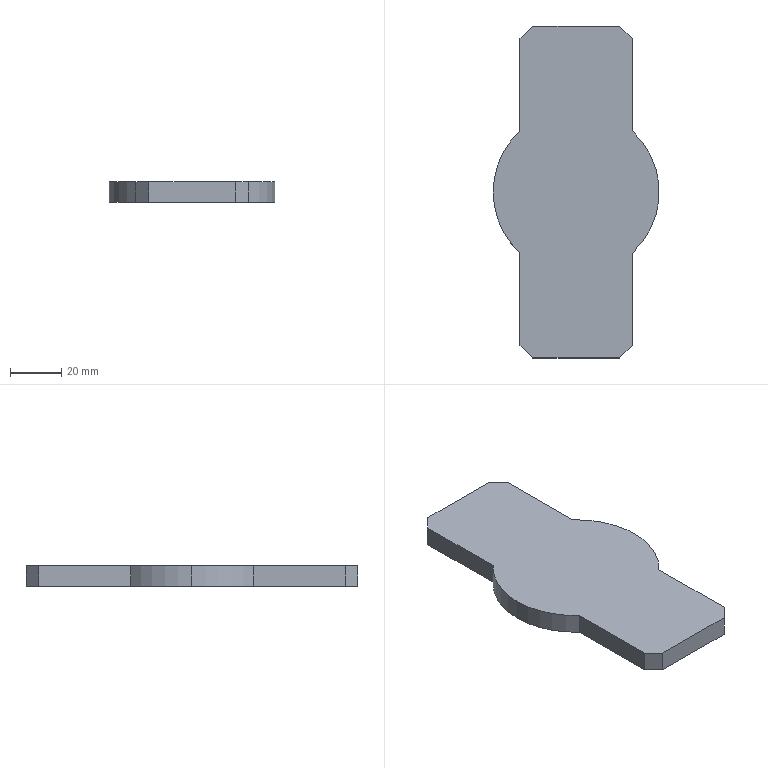Part | SolidWorks | features Chamfer 1, Extrusion 1, ICE 1 | 1 solid | 15 faces | box 65 x 130 x 8 mm | volume 50920 mm3 | plane 12 | cylinder 3 | commonest cylinder face diameters 65 x3
STEP:
#1=CARTESIAN_POINT('',(-32.5,0.,4.));
#2=VERTEX_POINT('',#1);
#3=CARTESIAN_POINT('',(-22.,-23.922,4.));
#4=VERTEX_POINT('',#3);
#5=CARTESIAN_POINT('',(0.,0.,4.));
#6=DIRECTION('',(0.,0.,1.));
#7=DIRECTION('',(1.,0.,0.));
#8=AXIS2_PLACEMENT_3D('',#5,#6,#7);
#9=CIRCLE('',#8,32.5);
#10=EDGE_CURVE('',#2,#4,#9,.T.);
#11=ORIENTED_EDGE('',*,*,#10,.F.);
#12=CARTESIAN_POINT('',(-32.5,0.,-4.));
#13=VERTEX_POINT('',#12);
#14=CARTESIAN_POINT('',(-32.5,0.,4.));
#15=DIRECTION('',(0.,0.,-1.));
#16=VECTOR('',#15,1000.);
#17=LINE('',#14,#16);
#18=EDGE_CURVE('',#2,#13,#17,.T.);
#19=ORIENTED_EDGE('',*,*,#18,.T.);
#20=CARTESIAN_POINT('',(-22.,-23.922,-4.));
#21=VERTEX_POINT('',#20);
#22=CARTESIAN_POINT('',(0.,0.,-4.));
#23=DIRECTION('',(0.,0.,1.));
#24=DIRECTION('',(1.,0.,0.));
#25=AXIS2_PLACEMENT_3D('',#22,#23,#24);
#26=CIRCLE('',#25,32.5);
#27=EDGE_CURVE('',#13,#21,#26,.T.);
#28=ORIENTED_EDGE('',*,*,#27,.T.);
#29=CARTESIAN_POINT('',(-22.,-23.922,4.));
#30=DIRECTION('',(0.,0.,1.));
#31=VECTOR('',#30,1000.);
#32=LINE('',#29,#31);
#33=EDGE_CURVE('',#21,#4,#32,.T.);
#34=ORIENTED_EDGE('',*,*,#33,.T.);
#35=EDGE_LOOP('',(#11,#19,#28,#34));
#36=FACE_OUTER_BOUND('',#35,.T.);
#37=CARTESIAN_POINT('',(0.,0.,4.));
#38=DIRECTION('',(0.,0.,-1.));
#39=DIRECTION('',(-1.,0.,0.));
#40=AXIS2_PLACEMENT_3D('',#37,#38,#39);
#41=CYLINDRICAL_SURFACE('',#40,32.5);
#42=ADVANCED_FACE('',(#36),#41,.T.);
#43=CARTESIAN_POINT('',(22.,-23.922,4.));
#44=VERTEX_POINT('',#43);
#45=CARTESIAN_POINT('',(22.,23.922,4.));
#46=VERTEX_POINT('',#45);
#47=CARTESIAN_POINT('',(0.,0.,4.));
#48=DIRECTION('',(0.,0.,1.));
#49=DIRECTION('',(1.,0.,0.));
#50=AXIS2_PLACEMENT_3D('',#47,#48,#49);
#51=CIRCLE('',#50,32.5);
#52=EDGE_CURVE('',#44,#46,#51,.T.);
#53=ORIENTED_EDGE('',*,*,#52,.F.);
#54=CARTESIAN_POINT('',(22.,-23.922,-4.));
#55=VERTEX_POINT('',#54);
#56=CARTESIAN_POINT('',(22.,-23.922,4.));
#57=DIRECTION('',(0.,0.,-1.));
#58=VECTOR('',#57,1000.);
#59=LINE('',#56,#58);
#60=EDGE_CURVE('',#44,#55,#59,.T.);
#61=ORIENTED_EDGE('',*,*,#60,.T.);
#62=CARTESIAN_POINT('',(22.,23.922,-4.));
#63=VERTEX_POINT('',#62);
#64=CARTESIAN_POINT('',(0.,0.,-4.));
#65=DIRECTION('',(0.,0.,1.));
#66=DIRECTION('',(1.,0.,0.));
#67=AXIS2_PLACEMENT_3D('',#64,#65,#66);
#68=CIRCLE('',#67,32.5);
#69=EDGE_CURVE('',#55,#63,#68,.T.);
#70=ORIENTED_EDGE('',*,*,#69,.T.);
#71=CARTESIAN_POINT('',(22.,23.922,4.));
#72=DIRECTION('',(0.,0.,1.));
#73=VECTOR('',#72,1000.);
#74=LINE('',#71,#73);
#75=EDGE_CURVE('',#63,#46,#74,.T.);
#76=ORIENTED_EDGE('',*,*,#75,.T.);
#77=EDGE_LOOP('',(#53,#61,#70,#76));
#78=FACE_OUTER_BOUND('',#77,.T.);
#79=CARTESIAN_POINT('',(0.,0.,4.));
#80=DIRECTION('',(0.,0.,-1.));
#81=DIRECTION('',(-1.,0.,0.));
#82=AXIS2_PLACEMENT_3D('',#79,#80,#81);
#83=CYLINDRICAL_SURFACE('',#82,32.5);
#84=ADVANCED_FACE('',(#78),#83,.T.);
#85=ORIENTED_EDGE('',*,*,#18,.F.);
#86=CARTESIAN_POINT('',(-22.,23.922,4.));
#87=VERTEX_POINT('',#86);
#88=CARTESIAN_POINT('',(0.,0.,4.));
#89=DIRECTION('',(0.,0.,1.));
#90=DIRECTION('',(1.,0.,0.));
#91=AXIS2_PLACEMENT_3D('',#88,#89,#90);
#92=CIRCLE('',#91,32.5);
#93=EDGE_CURVE('',#87,#2,#92,.T.);
#94=ORIENTED_EDGE('',*,*,#93,.F.);
#95=CARTESIAN_POINT('',(-22.,23.922,-4.));
#96=VERTEX_POINT('',#95);
#97=CARTESIAN_POINT('',(-22.,23.922,4.));
#98=DIRECTION('',(0.,0.,-1.));
#99=VECTOR('',#98,1000.);
#100=LINE('',#97,#99);
#101=EDGE_CURVE('',#87,#96,#100,.T.);
#102=ORIENTED_EDGE('',*,*,#101,.T.);
#103=CARTESIAN_POINT('',(0.,0.,-4.));
#104=DIRECTION('',(0.,0.,1.));
#105=DIRECTION('',(1.,0.,0.));
#106=AXIS2_PLACEMENT_3D('',#103,#104,#105);
#107=CIRCLE('',#106,32.5);
#108=EDGE_CURVE('',#96,#13,#107,.T.);
#109=ORIENTED_EDGE('',*,*,#108,.T.);
#110=EDGE_LOOP('',(#85,#94,#102,#109));
#111=FACE_OUTER_BOUND('',#110,.T.);
#112=CARTESIAN_POINT('',(0.,0.,4.));
#113=DIRECTION('',(0.,0.,-1.));
#114=DIRECTION('',(-1.,0.,0.));
#115=AXIS2_PLACEMENT_3D('',#112,#113,#114);
#116=CYLINDRICAL_SURFACE('',#115,32.5);
#117=ADVANCED_FACE('',(#111),#116,.T.);
#118=CARTESIAN_POINT('',(-17.,-65.,4.));
#119=VERTEX_POINT('',#118);
#120=CARTESIAN_POINT('',(17.,-65.,4.));
#121=VERTEX_POINT('',#120);
#122=CARTESIAN_POINT('',(-22.,-65.,4.));
#123=DIRECTION('',(1.,0.,0.));
#124=VECTOR('',#123,1000.);
#125=LINE('',#122,#124);
#126=EDGE_CURVE('',#119,#121,#125,.T.);
#127=ORIENTED_EDGE('',*,*,#126,.T.);
#128=CARTESIAN_POINT('',(22.,-60.,4.));
#129=VERTEX_POINT('',#128);
#130=CARTESIAN_POINT('',(41.,-41.,4.));
#131=DIRECTION('',(0.7071,0.7071,0.));
#132=VECTOR('',#131,1000.);
#133=LINE('',#130,#132);
#134=EDGE_CURVE('',#121,#129,#133,.T.);
#135=ORIENTED_EDGE('',*,*,#134,.T.);
#136=CARTESIAN_POINT('',(22.,65.,4.));
#137=DIRECTION('',(0.,1.,0.));
#138=VECTOR('',#137,1000.);
#139=LINE('',#136,#138);
#140=EDGE_CURVE('',#129,#44,#139,.T.);
#141=ORIENTED_EDGE('',*,*,#140,.T.);
#142=ORIENTED_EDGE('',*,*,#52,.T.);
#143=CARTESIAN_POINT('',(22.,60.,4.));
#144=VERTEX_POINT('',#143);
#145=CARTESIAN_POINT('',(22.,65.,4.));
#146=DIRECTION('',(0.,1.,0.));
#147=VECTOR('',#146,1000.);
#148=LINE('',#145,#147);
#149=EDGE_CURVE('',#46,#144,#148,.T.);
#150=ORIENTED_EDGE('',*,*,#149,.T.);
#151=CARTESIAN_POINT('',(17.,65.,4.));
#152=VERTEX_POINT('',#151);
#153=CARTESIAN_POINT('',(41.,41.,4.));
#154=DIRECTION('',(-0.7071,0.7071,0.));
#155=VECTOR('',#154,1000.);
#156=LINE('',#153,#155);
#157=EDGE_CURVE('',#144,#152,#156,.T.);
#158=ORIENTED_EDGE('',*,*,#157,.T.);
#159=CARTESIAN_POINT('',(-17.,65.,4.));
#160=VERTEX_POINT('',#159);
#161=CARTESIAN_POINT('',(-22.,65.,4.));
#162=DIRECTION('',(-1.,0.,0.));
#163=VECTOR('',#162,1000.);
#164=LINE('',#161,#163);
#165=EDGE_CURVE('',#152,#160,#164,.T.);
#166=ORIENTED_EDGE('',*,*,#165,.T.);
#167=CARTESIAN_POINT('',(-22.,60.,4.));
#168=VERTEX_POINT('',#167);
#169=CARTESIAN_POINT('',(-41.,41.,4.));
#170=DIRECTION('',(-0.7071,-0.7071,0.));
#171=VECTOR('',#170,1000.);
#172=LINE('',#169,#171);
#173=EDGE_CURVE('',#160,#168,#172,.T.);
#174=ORIENTED_EDGE('',*,*,#173,.T.);
#175=CARTESIAN_POINT('',(-22.,65.,4.));
#176=DIRECTION('',(0.,-1.,0.));
#177=VECTOR('',#176,1000.);
#178=LINE('',#175,#177);
#179=EDGE_CURVE('',#168,#87,#178,.T.);
#180=ORIENTED_EDGE('',*,*,#179,.T.);
#181=ORIENTED_EDGE('',*,*,#93,.T.);
#182=ORIENTED_EDGE('',*,*,#10,.T.);
#183=CARTESIAN_POINT('',(-22.,-60.,4.));
#184=VERTEX_POINT('',#183);
#185=CARTESIAN_POINT('',(-22.,65.,4.));
#186=DIRECTION('',(0.,-1.,0.));
#187=VECTOR('',#186,1000.);
#188=LINE('',#185,#187);
#189=EDGE_CURVE('',#4,#184,#188,.T.);
#190=ORIENTED_EDGE('',*,*,#189,.T.);
#191=CARTESIAN_POINT('',(-41.,-41.,4.));
#192=DIRECTION('',(0.7071,-0.7071,0.));
#193=VECTOR('',#192,1000.);
#194=LINE('',#191,#193);
#195=EDGE_CURVE('',#184,#119,#194,.T.);
#196=ORIENTED_EDGE('',*,*,#195,.T.);
#197=EDGE_LOOP('',(#127,#135,#141,#142,#150,#158,#166,#174,#180,#181,#182,#190,#196));
#198=FACE_OUTER_BOUND('',#197,.T.);
#199=CARTESIAN_POINT('',(0.,0.,4.));
#200=DIRECTION('',(0.,0.,1.));
#201=DIRECTION('',(1.,0.,0.));
#202=AXIS2_PLACEMENT_3D('',#199,#200,#201);
#203=PLANE('',#202);
#204=ADVANCED_FACE('',(#198),#203,.T.);
#205=CARTESIAN_POINT('',(22.,-60.,-4.));
#206=VERTEX_POINT('',#205);
#207=CARTESIAN_POINT('',(22.,65.,-4.));
#208=DIRECTION('',(0.,-1.,0.));
#209=VECTOR('',#208,1000.);
#210=LINE('',#207,#209);
#211=EDGE_CURVE('',#55,#206,#210,.T.);
#212=ORIENTED_EDGE('',*,*,#211,.T.);
#213=CARTESIAN_POINT('',(17.,-65.,-4.));
#214=VERTEX_POINT('',#213);
#215=CARTESIAN_POINT('',(17.,-65.,-4.));
#216=DIRECTION('',(-0.7071,-0.7071,0.));
#217=VECTOR('',#216,1000.);
#218=LINE('',#215,#217);
#219=EDGE_CURVE('',#206,#214,#218,.T.);
#220=ORIENTED_EDGE('',*,*,#219,.T.);
#221=CARTESIAN_POINT('',(-17.,-65.,-4.));
#222=VERTEX_POINT('',#221);
#223=CARTESIAN_POINT('',(-22.,-65.,-4.));
#224=DIRECTION('',(-1.,0.,0.));
#225=VECTOR('',#224,1000.);
#226=LINE('',#223,#225);
#227=EDGE_CURVE('',#214,#222,#226,.T.);
#228=ORIENTED_EDGE('',*,*,#227,.T.);
#229=CARTESIAN_POINT('',(-22.,-60.,-4.));
#230=VERTEX_POINT('',#229);
#231=CARTESIAN_POINT('',(-22.,-60.,-4.));
#232=DIRECTION('',(-0.7071,0.7071,0.));
#233=VECTOR('',#232,1000.);
#234=LINE('',#231,#233);
#235=EDGE_CURVE('',#222,#230,#234,.T.);
#236=ORIENTED_EDGE('',*,*,#235,.T.);
#237=CARTESIAN_POINT('',(-22.,65.,-4.));
#238=DIRECTION('',(0.,1.,0.));
#239=VECTOR('',#238,1000.);
#240=LINE('',#237,#239);
#241=EDGE_CURVE('',#230,#21,#240,.T.);
#242=ORIENTED_EDGE('',*,*,#241,.T.);
#243=ORIENTED_EDGE('',*,*,#27,.F.);
#244=ORIENTED_EDGE('',*,*,#108,.F.);
#245=CARTESIAN_POINT('',(-22.,60.,-4.));
#246=VERTEX_POINT('',#245);
#247=CARTESIAN_POINT('',(-22.,65.,-4.));
#248=DIRECTION('',(0.,1.,0.));
#249=VECTOR('',#248,1000.);
#250=LINE('',#247,#249);
#251=EDGE_CURVE('',#96,#246,#250,.T.);
#252=ORIENTED_EDGE('',*,*,#251,.T.);
#253=CARTESIAN_POINT('',(-17.,65.,-4.));
#254=VERTEX_POINT('',#253);
#255=CARTESIAN_POINT('',(-17.,65.,-4.));
#256=DIRECTION('',(0.7071,0.7071,0.));
#257=VECTOR('',#256,1000.);
#258=LINE('',#255,#257);
#259=EDGE_CURVE('',#246,#254,#258,.T.);
#260=ORIENTED_EDGE('',*,*,#259,.T.);
#261=CARTESIAN_POINT('',(17.,65.,-4.));
#262=VERTEX_POINT('',#261);
#263=CARTESIAN_POINT('',(-22.,65.,-4.));
#264=DIRECTION('',(1.,0.,0.));
#265=VECTOR('',#264,1000.);
#266=LINE('',#263,#265);
#267=EDGE_CURVE('',#254,#262,#266,.T.);
#268=ORIENTED_EDGE('',*,*,#267,.T.);
#269=CARTESIAN_POINT('',(22.,60.,-4.));
#270=VERTEX_POINT('',#269);
#271=CARTESIAN_POINT('',(22.,60.,-4.));
#272=DIRECTION('',(0.7071,-0.7071,0.));
#273=VECTOR('',#272,1000.);
#274=LINE('',#271,#273);
#275=EDGE_CURVE('',#262,#270,#274,.T.);
#276=ORIENTED_EDGE('',*,*,#275,.T.);
#277=CARTESIAN_POINT('',(22.,65.,-4.));
#278=DIRECTION('',(0.,-1.,0.));
#279=VECTOR('',#278,1000.);
#280=LINE('',#277,#279);
#281=EDGE_CURVE('',#270,#63,#280,.T.);
#282=ORIENTED_EDGE('',*,*,#281,.T.);
#283=ORIENTED_EDGE('',*,*,#69,.F.);
#284=EDGE_LOOP('',(#212,#220,#228,#236,#242,#243,#244,#252,#260,#268,#276,#282,#283));
#285=FACE_OUTER_BOUND('',#284,.T.);
#286=CARTESIAN_POINT('',(0.,0.,-4.));
#287=DIRECTION('',(0.,0.,1.));
#288=DIRECTION('',(1.,0.,0.));
#289=AXIS2_PLACEMENT_3D('',#286,#287,#288);
#290=PLANE('',#289);
#291=ADVANCED_FACE('',(#285),#290,.F.);
#292=ORIENTED_EDGE('',*,*,#227,.F.);
#293=CARTESIAN_POINT('',(17.,-65.,-141.244));
#294=DIRECTION('',(0.,0.,1.));
#295=VECTOR('',#294,1000.);
#296=LINE('',#293,#295);
#297=EDGE_CURVE('',#214,#121,#296,.T.);
#298=ORIENTED_EDGE('',*,*,#297,.T.);
#299=ORIENTED_EDGE('',*,*,#126,.F.);
#300=CARTESIAN_POINT('',(-17.,-65.,-141.244));
#301=DIRECTION('',(0.,0.,-1.));
#302=VECTOR('',#301,1000.);
#303=LINE('',#300,#302);
#304=EDGE_CURVE('',#119,#222,#303,.T.);
#305=ORIENTED_EDGE('',*,*,#304,.T.);
#306=EDGE_LOOP('',(#292,#298,#299,#305));
#307=FACE_OUTER_BOUND('',#306,.T.);
#308=CARTESIAN_POINT('',(-22.,-65.,-141.244));
#309=DIRECTION('',(0.,-1.,0.));
#310=DIRECTION('',(0.,0.,-1.));
#311=AXIS2_PLACEMENT_3D('',#308,#309,#310);
#312=PLANE('',#311);
#313=ADVANCED_FACE('',(#307),#312,.T.);
#314=ORIENTED_EDGE('',*,*,#241,.F.);
#315=CARTESIAN_POINT('',(-22.,-60.,-141.244));
#316=DIRECTION('',(0.,0.,1.));
#317=VECTOR('',#316,1000.);
#318=LINE('',#315,#317);
#319=EDGE_CURVE('',#230,#184,#318,.T.);
#320=ORIENTED_EDGE('',*,*,#319,.T.);
#321=ORIENTED_EDGE('',*,*,#189,.F.);
#322=ORIENTED_EDGE('',*,*,#33,.F.);
#323=EDGE_LOOP('',(#314,#320,#321,#322));
#324=FACE_OUTER_BOUND('',#323,.T.);
#325=CARTESIAN_POINT('',(-22.,65.,-141.244));
#326=DIRECTION('',(-1.,0.,0.));
#327=DIRECTION('',(0.,-1.,0.));
#328=AXIS2_PLACEMENT_3D('',#325,#326,#327);
#329=PLANE('',#328);
#330=ADVANCED_FACE('',(#324),#329,.T.);
#331=ORIENTED_EDGE('',*,*,#140,.F.);
#332=CARTESIAN_POINT('',(22.,-60.,-141.244));
#333=DIRECTION('',(0.,0.,-1.));
#334=VECTOR('',#333,1000.);
#335=LINE('',#332,#334);
#336=EDGE_CURVE('',#129,#206,#335,.T.);
#337=ORIENTED_EDGE('',*,*,#336,.T.);
#338=ORIENTED_EDGE('',*,*,#211,.F.);
#339=ORIENTED_EDGE('',*,*,#60,.F.);
#340=EDGE_LOOP('',(#331,#337,#338,#339));
#341=FACE_OUTER_BOUND('',#340,.T.);
#342=CARTESIAN_POINT('',(22.,65.,-141.244));
#343=DIRECTION('',(1.,0.,0.));
#344=DIRECTION('',(0.,1.,0.));
#345=AXIS2_PLACEMENT_3D('',#342,#343,#344);
#346=PLANE('',#345);
#347=ADVANCED_FACE('',(#341),#346,.T.);
#348=ORIENTED_EDGE('',*,*,#281,.F.);
#349=CARTESIAN_POINT('',(22.,60.,-141.244));
#350=DIRECTION('',(0.,0.,1.));
#351=VECTOR('',#350,1000.);
#352=LINE('',#349,#351);
#353=EDGE_CURVE('',#270,#144,#352,.T.);
#354=ORIENTED_EDGE('',*,*,#353,.T.);
#355=ORIENTED_EDGE('',*,*,#149,.F.);
#356=ORIENTED_EDGE('',*,*,#75,.F.);
#357=EDGE_LOOP('',(#348,#354,#355,#356));
#358=FACE_OUTER_BOUND('',#357,.T.);
#359=CARTESIAN_POINT('',(22.,65.,-141.244));
#360=DIRECTION('',(1.,0.,0.));
#361=DIRECTION('',(0.,1.,0.));
#362=AXIS2_PLACEMENT_3D('',#359,#360,#361);
#363=PLANE('',#362);
#364=ADVANCED_FACE('',(#358),#363,.T.);
#365=ORIENTED_EDGE('',*,*,#179,.F.);
#366=CARTESIAN_POINT('',(-22.,60.,-141.244));
#367=DIRECTION('',(0.,0.,-1.));
#368=VECTOR('',#367,1000.);
#369=LINE('',#366,#368);
#370=EDGE_CURVE('',#168,#246,#369,.T.);
#371=ORIENTED_EDGE('',*,*,#370,.T.);
#372=ORIENTED_EDGE('',*,*,#251,.F.);
#373=ORIENTED_EDGE('',*,*,#101,.F.);
#374=EDGE_LOOP('',(#365,#371,#372,#373));
#375=FACE_OUTER_BOUND('',#374,.T.);
#376=CARTESIAN_POINT('',(-22.,65.,-141.244));
#377=DIRECTION('',(-1.,0.,0.));
#378=DIRECTION('',(0.,-1.,0.));
#379=AXIS2_PLACEMENT_3D('',#376,#377,#378);
#380=PLANE('',#379);
#381=ADVANCED_FACE('',(#375),#380,.T.);
#382=ORIENTED_EDGE('',*,*,#165,.F.);
#383=CARTESIAN_POINT('',(17.,65.,-141.244));
#384=DIRECTION('',(0.,0.,-1.));
#385=VECTOR('',#384,1000.);
#386=LINE('',#383,#385);
#387=EDGE_CURVE('',#152,#262,#386,.T.);
#388=ORIENTED_EDGE('',*,*,#387,.T.);
#389=ORIENTED_EDGE('',*,*,#267,.F.);
#390=CARTESIAN_POINT('',(-17.,65.,-141.244));
#391=DIRECTION('',(0.,0.,1.));
#392=VECTOR('',#391,1000.);
#393=LINE('',#390,#392);
#394=EDGE_CURVE('',#254,#160,#393,.T.);
#395=ORIENTED_EDGE('',*,*,#394,.T.);
#396=EDGE_LOOP('',(#382,#388,#389,#395));
#397=FACE_OUTER_BOUND('',#396,.T.);
#398=CARTESIAN_POINT('',(-22.,65.,-141.244));
#399=DIRECTION('',(0.,1.,0.));
#400=DIRECTION('',(0.,0.,1.));
#401=AXIS2_PLACEMENT_3D('',#398,#399,#400);
#402=PLANE('',#401);
#403=ADVANCED_FACE('',(#397),#402,.T.);
#404=ORIENTED_EDGE('',*,*,#219,.F.);
#405=ORIENTED_EDGE('',*,*,#336,.F.);
#406=ORIENTED_EDGE('',*,*,#134,.F.);
#407=ORIENTED_EDGE('',*,*,#297,.F.);
#408=EDGE_LOOP('',(#404,#405,#406,#407));
#409=FACE_OUTER_BOUND('',#408,.T.);
#410=CARTESIAN_POINT('',(17.,-65.,-141.244));
#411=DIRECTION('',(-0.7071,0.7071,0.));
#412=DIRECTION('',(0.,0.,1.));
#413=AXIS2_PLACEMENT_3D('',#410,#411,#412);
#414=PLANE('',#413);
#415=ADVANCED_FACE('',(#409),#414,.F.);
#416=ORIENTED_EDGE('',*,*,#275,.F.);
#417=ORIENTED_EDGE('',*,*,#387,.F.);
#418=ORIENTED_EDGE('',*,*,#157,.F.);
#419=ORIENTED_EDGE('',*,*,#353,.F.);
#420=EDGE_LOOP('',(#416,#417,#418,#419));
#421=FACE_OUTER_BOUND('',#420,.T.);
#422=CARTESIAN_POINT('',(22.,60.,-141.244));
#423=DIRECTION('',(-0.7071,-0.7071,0.));
#424=DIRECTION('',(0.,0.,1.));
#425=AXIS2_PLACEMENT_3D('',#422,#423,#424);
#426=PLANE('',#425);
#427=ADVANCED_FACE('',(#421),#426,.F.);
#428=ORIENTED_EDGE('',*,*,#235,.F.);
#429=ORIENTED_EDGE('',*,*,#304,.F.);
#430=ORIENTED_EDGE('',*,*,#195,.F.);
#431=ORIENTED_EDGE('',*,*,#319,.F.);
#432=EDGE_LOOP('',(#428,#429,#430,#431));
#433=FACE_OUTER_BOUND('',#432,.T.);
#434=CARTESIAN_POINT('',(-22.,-60.,-141.244));
#435=DIRECTION('',(0.7071,0.7071,0.));
#436=DIRECTION('',(0.,0.,1.));
#437=AXIS2_PLACEMENT_3D('',#434,#435,#436);
#438=PLANE('',#437);
#439=ADVANCED_FACE('',(#433),#438,.F.);
#440=ORIENTED_EDGE('',*,*,#259,.F.);
#441=ORIENTED_EDGE('',*,*,#370,.F.);
#442=ORIENTED_EDGE('',*,*,#173,.F.);
#443=ORIENTED_EDGE('',*,*,#394,.F.);
#444=EDGE_LOOP('',(#440,#441,#442,#443));
#445=FACE_OUTER_BOUND('',#444,.T.);
#446=CARTESIAN_POINT('',(-17.,65.,-141.244));
#447=DIRECTION('',(0.7071,-0.7071,0.));
#448=DIRECTION('',(0.,0.,1.));
#449=AXIS2_PLACEMENT_3D('',#446,#447,#448);
#450=PLANE('',#449);
#451=ADVANCED_FACE('',(#445),#450,.F.);
#452=CLOSED_SHELL('',(#42,#84,#117,#204,#291,#313,#330,#347,#364,#381,#403,#415,#427,#439,#451));
#453=MANIFOLD_SOLID_BREP('',#452);
#454=CARTESIAN_POINT('',(0.,0.,0.));
#455=DIRECTION('',(0.,0.,1.));
#456=DIRECTION('',(1.,0.,0.));
#457=AXIS2_PLACEMENT_3D('',#454,#455,#456);
#458=(LENGTH_UNIT()NAMED_UNIT(*)SI_UNIT(.MILLI.,.METRE.));
#459=UNCERTAINTY_MEASURE_WITH_UNIT(LENGTH_MEASURE(0.00001),#458,'','');
#460=(NAMED_UNIT(*)PLANE_ANGLE_UNIT()SI_UNIT($,.RADIAN.));
#461=(NAMED_UNIT(*)SI_UNIT($,.STERADIAN.)SOLID_ANGLE_UNIT());
#462=(GEOMETRIC_REPRESENTATION_CONTEXT(3)GLOBAL_UNCERTAINTY_ASSIGNED_CONTEXT((#459))GLOBAL_UNIT_ASSIGNED_CONTEXT((#458,#460,#461))REPRESENTATION_CONTEXT('',''));
#463=ADVANCED_BREP_SHAPE_REPRESENTATION('',(#453,#457),#462);